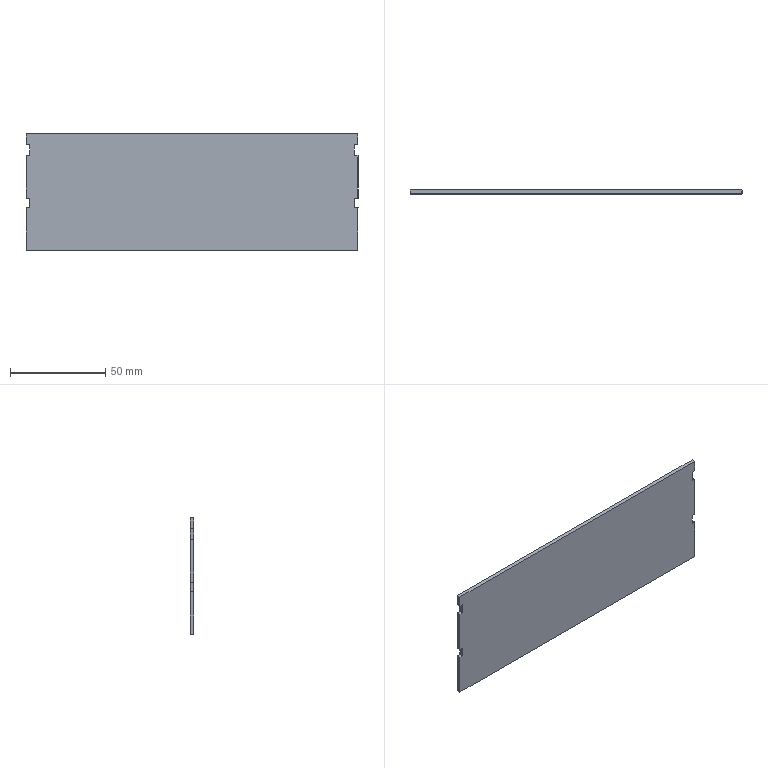Part | SolidWorks | features MirrorStock 1 | 1 solid | 22 faces | box 174 x 2 x 61 mm | volume 21144 mm3 | plane 22
STEP:
#1=CARTESIAN_POINT('',(-87.,-39.2,-39.75));
#2=VERTEX_POINT('',#1);
#3=CARTESIAN_POINT('',(-87.,-41.2,-39.75));
#4=VERTEX_POINT('',#3);
#5=CARTESIAN_POINT('',(-87.,-40.2,-39.75));
#6=DIRECTION('',(0.,-1.,0.));
#7=VECTOR('',#6,1000.);
#8=LINE('',#5,#7);
#9=EDGE_CURVE('',#2,#4,#8,.T.);
#10=ORIENTED_EDGE('',*,*,#9,.T.);
#11=CARTESIAN_POINT('',(-85.,-41.2,-39.75));
#12=VERTEX_POINT('',#11);
#13=CARTESIAN_POINT('',(0.,-41.2,-39.75));
#14=DIRECTION('',(1.,0.,0.));
#15=VECTOR('',#14,1000.);
#16=LINE('',#13,#15);
#17=EDGE_CURVE('',#4,#12,#16,.T.);
#18=ORIENTED_EDGE('',*,*,#17,.T.);
#19=CARTESIAN_POINT('',(-85.,-39.2,-39.75));
#20=VERTEX_POINT('',#19);
#21=CARTESIAN_POINT('',(-85.,-40.2,-39.75));
#22=DIRECTION('',(0.,1.,0.));
#23=VECTOR('',#22,1000.);
#24=LINE('',#21,#23);
#25=EDGE_CURVE('',#12,#20,#24,.T.);
#26=ORIENTED_EDGE('',*,*,#25,.T.);
#27=CARTESIAN_POINT('',(0.,-39.2,-39.75));
#28=DIRECTION('',(-1.,0.,0.));
#29=VECTOR('',#28,1000.);
#30=LINE('',#27,#29);
#31=EDGE_CURVE('',#20,#2,#30,.T.);
#32=ORIENTED_EDGE('',*,*,#31,.T.);
#33=EDGE_LOOP('',(#10,#18,#26,#32));
#34=FACE_OUTER_BOUND('',#33,.T.);
#35=CARTESIAN_POINT('',(-84.779,-38.979,-39.75));
#36=DIRECTION('',(0.,0.,1.));
#37=DIRECTION('',(0.,-1.,0.));
#38=AXIS2_PLACEMENT_3D('',#35,#36,#37);
#39=PLANE('',#38);
#40=ADVANCED_FACE('',(#34),#39,.T.);
#41=CARTESIAN_POINT('',(-85.,-41.2,-34.75));
#42=VERTEX_POINT('',#41);
#43=CARTESIAN_POINT('',(-85.,-39.2,-34.75));
#44=VERTEX_POINT('',#43);
#45=CARTESIAN_POINT('',(-85.,-40.2,-34.75));
#46=DIRECTION('',(0.,1.,0.));
#47=VECTOR('',#46,1000.);
#48=LINE('',#45,#47);
#49=EDGE_CURVE('',#42,#44,#48,.T.);
#50=ORIENTED_EDGE('',*,*,#49,.T.);
#51=CARTESIAN_POINT('',(-85.,-39.2,-31.5));
#52=DIRECTION('',(0.,0.,-1.));
#53=VECTOR('',#52,1000.);
#54=LINE('',#51,#53);
#55=EDGE_CURVE('',#44,#20,#54,.T.);
#56=ORIENTED_EDGE('',*,*,#55,.T.);
#57=ORIENTED_EDGE('',*,*,#25,.F.);
#58=CARTESIAN_POINT('',(-85.,-41.2,-31.5));
#59=DIRECTION('',(0.,0.,1.));
#60=VECTOR('',#59,1000.);
#61=LINE('',#58,#60);
#62=EDGE_CURVE('',#12,#42,#61,.T.);
#63=ORIENTED_EDGE('',*,*,#62,.T.);
#64=EDGE_LOOP('',(#50,#56,#57,#63));
#65=FACE_OUTER_BOUND('',#64,.T.);
#66=CARTESIAN_POINT('',(-85.,-41.421,-34.529));
#67=DIRECTION('',(-1.,0.,0.));
#68=DIRECTION('',(0.,0.,-1.));
#69=AXIS2_PLACEMENT_3D('',#66,#67,#68);
#70=PLANE('',#69);
#71=ADVANCED_FACE('',(#65),#70,.T.);
#72=CARTESIAN_POINT('',(-87.,-41.2,-34.75));
#73=VERTEX_POINT('',#72);
#74=CARTESIAN_POINT('',(-87.,-39.2,-34.75));
#75=VERTEX_POINT('',#74);
#76=CARTESIAN_POINT('',(-87.,-40.2,-34.75));
#77=DIRECTION('',(0.,1.,0.));
#78=VECTOR('',#77,1000.);
#79=LINE('',#76,#78);
#80=EDGE_CURVE('',#73,#75,#79,.T.);
#81=ORIENTED_EDGE('',*,*,#80,.T.);
#82=CARTESIAN_POINT('',(0.,-39.2,-34.75));
#83=DIRECTION('',(1.,0.,0.));
#84=VECTOR('',#83,1000.);
#85=LINE('',#82,#84);
#86=EDGE_CURVE('',#75,#44,#85,.T.);
#87=ORIENTED_EDGE('',*,*,#86,.T.);
#88=ORIENTED_EDGE('',*,*,#49,.F.);
#89=CARTESIAN_POINT('',(0.,-41.2,-34.75));
#90=DIRECTION('',(-1.,0.,0.));
#91=VECTOR('',#90,1000.);
#92=LINE('',#89,#91);
#93=EDGE_CURVE('',#42,#73,#92,.T.);
#94=ORIENTED_EDGE('',*,*,#93,.T.);
#95=EDGE_LOOP('',(#81,#87,#88,#94));
#96=FACE_OUTER_BOUND('',#95,.T.);
#97=CARTESIAN_POINT('',(-84.779,-41.421,-34.75));
#98=DIRECTION('',(0.,0.,-1.));
#99=DIRECTION('',(0.,1.,0.));
#100=AXIS2_PLACEMENT_3D('',#97,#98,#99);
#101=PLANE('',#100);
#102=ADVANCED_FACE('',(#96),#101,.T.);
#103=CARTESIAN_POINT('',(-87.,-41.2,-12.25));
#104=VERTEX_POINT('',#103);
#105=CARTESIAN_POINT('',(-87.,-39.2,-12.25));
#106=VERTEX_POINT('',#105);
#107=CARTESIAN_POINT('',(-87.,-40.2,-12.25));
#108=DIRECTION('',(0.,1.,0.));
#109=VECTOR('',#108,1000.);
#110=LINE('',#107,#109);
#111=EDGE_CURVE('',#104,#106,#110,.T.);
#112=ORIENTED_EDGE('',*,*,#111,.T.);
#113=CARTESIAN_POINT('',(-87.,-39.2,-31.5));
#114=DIRECTION('',(0.,0.,-1.));
#115=VECTOR('',#114,1000.);
#116=LINE('',#113,#115);
#117=EDGE_CURVE('',#106,#75,#116,.T.);
#118=ORIENTED_EDGE('',*,*,#117,.T.);
#119=ORIENTED_EDGE('',*,*,#80,.F.);
#120=CARTESIAN_POINT('',(-87.,-41.2,-31.5));
#121=DIRECTION('',(0.,0.,1.));
#122=VECTOR('',#121,1000.);
#123=LINE('',#120,#122);
#124=EDGE_CURVE('',#73,#104,#123,.T.);
#125=ORIENTED_EDGE('',*,*,#124,.T.);
#126=EDGE_LOOP('',(#112,#118,#119,#125));
#127=FACE_OUTER_BOUND('',#126,.T.);
#128=CARTESIAN_POINT('',(-87.,-41.421,-63.22));
#129=DIRECTION('',(-1.,0.,0.));
#130=DIRECTION('',(0.,1.,0.));
#131=AXIS2_PLACEMENT_3D('',#128,#129,#130);
#132=PLANE('',#131);
#133=ADVANCED_FACE('',(#127),#132,.T.);
#134=CARTESIAN_POINT('',(-85.,-41.2,-12.25));
#135=VERTEX_POINT('',#134);
#136=CARTESIAN_POINT('',(-85.,-39.2,-12.25));
#137=VERTEX_POINT('',#136);
#138=CARTESIAN_POINT('',(-85.,-40.2,-12.25));
#139=DIRECTION('',(0.,1.,0.));
#140=VECTOR('',#139,1000.);
#141=LINE('',#138,#140);
#142=EDGE_CURVE('',#135,#137,#141,.T.);
#143=ORIENTED_EDGE('',*,*,#142,.T.);
#144=CARTESIAN_POINT('',(0.,-39.2,-12.25));
#145=DIRECTION('',(-1.,0.,0.));
#146=VECTOR('',#145,1000.);
#147=LINE('',#144,#146);
#148=EDGE_CURVE('',#137,#106,#147,.T.);
#149=ORIENTED_EDGE('',*,*,#148,.T.);
#150=ORIENTED_EDGE('',*,*,#111,.F.);
#151=CARTESIAN_POINT('',(0.,-41.2,-12.25));
#152=DIRECTION('',(1.,0.,0.));
#153=VECTOR('',#152,1000.);
#154=LINE('',#151,#153);
#155=EDGE_CURVE('',#104,#135,#154,.T.);
#156=ORIENTED_EDGE('',*,*,#155,.T.);
#157=EDGE_LOOP('',(#143,#149,#150,#156));
#158=FACE_OUTER_BOUND('',#157,.T.);
#159=CARTESIAN_POINT('',(-84.779,-38.979,-12.25));
#160=DIRECTION('',(0.,0.,1.));
#161=DIRECTION('',(0.,-1.,0.));
#162=AXIS2_PLACEMENT_3D('',#159,#160,#161);
#163=PLANE('',#162);
#164=ADVANCED_FACE('',(#158),#163,.T.);
#165=CARTESIAN_POINT('',(-85.,-41.2,-6.75));
#166=VERTEX_POINT('',#165);
#167=CARTESIAN_POINT('',(-85.,-41.2,-31.5));
#168=DIRECTION('',(0.,0.,1.));
#169=VECTOR('',#168,1000.);
#170=LINE('',#167,#169);
#171=EDGE_CURVE('',#135,#166,#170,.T.);
#172=ORIENTED_EDGE('',*,*,#171,.T.);
#173=CARTESIAN_POINT('',(-85.,-39.2,-6.75));
#174=VERTEX_POINT('',#173);
#175=CARTESIAN_POINT('',(-85.,-40.2,-6.75));
#176=DIRECTION('',(0.,1.,0.));
#177=VECTOR('',#176,1000.);
#178=LINE('',#175,#177);
#179=EDGE_CURVE('',#166,#174,#178,.T.);
#180=ORIENTED_EDGE('',*,*,#179,.T.);
#181=CARTESIAN_POINT('',(-85.,-39.2,-31.5));
#182=DIRECTION('',(0.,0.,-1.));
#183=VECTOR('',#182,1000.);
#184=LINE('',#181,#183);
#185=EDGE_CURVE('',#174,#137,#184,.T.);
#186=ORIENTED_EDGE('',*,*,#185,.T.);
#187=ORIENTED_EDGE('',*,*,#142,.F.);
#188=EDGE_LOOP('',(#172,#180,#186,#187));
#189=FACE_OUTER_BOUND('',#188,.T.);
#190=CARTESIAN_POINT('',(-85.,-41.421,-6.529));
#191=DIRECTION('',(-1.,0.,0.));
#192=DIRECTION('',(0.,0.,-1.));
#193=AXIS2_PLACEMENT_3D('',#190,#191,#192);
#194=PLANE('',#193);
#195=ADVANCED_FACE('',(#189),#194,.T.);
#196=ORIENTED_EDGE('',*,*,#179,.F.);
#197=CARTESIAN_POINT('',(-87.,-41.2,-6.75));
#198=VERTEX_POINT('',#197);
#199=CARTESIAN_POINT('',(0.,-41.2,-6.75));
#200=DIRECTION('',(-1.,0.,0.));
#201=VECTOR('',#200,1000.);
#202=LINE('',#199,#201);
#203=EDGE_CURVE('',#166,#198,#202,.T.);
#204=ORIENTED_EDGE('',*,*,#203,.T.);
#205=CARTESIAN_POINT('',(-87.,-39.2,-6.75));
#206=VERTEX_POINT('',#205);
#207=CARTESIAN_POINT('',(-87.,-40.2,-6.75));
#208=DIRECTION('',(0.,1.,0.));
#209=VECTOR('',#208,1000.);
#210=LINE('',#207,#209);
#211=EDGE_CURVE('',#198,#206,#210,.T.);
#212=ORIENTED_EDGE('',*,*,#211,.T.);
#213=CARTESIAN_POINT('',(0.,-39.2,-6.75));
#214=DIRECTION('',(1.,0.,0.));
#215=VECTOR('',#214,1000.);
#216=LINE('',#213,#215);
#217=EDGE_CURVE('',#206,#174,#216,.T.);
#218=ORIENTED_EDGE('',*,*,#217,.T.);
#219=EDGE_LOOP('',(#196,#204,#212,#218));
#220=FACE_OUTER_BOUND('',#219,.T.);
#221=CARTESIAN_POINT('',(-84.779,-41.421,-6.75));
#222=DIRECTION('',(0.,0.,-1.));
#223=DIRECTION('',(0.,1.,0.));
#224=AXIS2_PLACEMENT_3D('',#221,#222,#223);
#225=PLANE('',#224);
#226=ADVANCED_FACE('',(#220),#225,.T.);
#227=CARTESIAN_POINT('',(87.,-41.2,-6.75));
#228=VERTEX_POINT('',#227);
#229=CARTESIAN_POINT('',(85.,-41.2,-6.75));
#230=VERTEX_POINT('',#229);
#231=CARTESIAN_POINT('',(0.,-41.2,-6.75));
#232=DIRECTION('',(-1.,0.,0.));
#233=VECTOR('',#232,1000.);
#234=LINE('',#231,#233);
#235=EDGE_CURVE('',#228,#230,#234,.T.);
#236=ORIENTED_EDGE('',*,*,#235,.T.);
#237=CARTESIAN_POINT('',(85.,-39.2,-6.75));
#238=VERTEX_POINT('',#237);
#239=CARTESIAN_POINT('',(85.,-40.2,-6.75));
#240=DIRECTION('',(0.,-1.,0.));
#241=VECTOR('',#240,1000.);
#242=LINE('',#239,#241);
#243=EDGE_CURVE('',#238,#230,#242,.T.);
#244=ORIENTED_EDGE('',*,*,#243,.F.);
#245=CARTESIAN_POINT('',(87.,-39.2,-6.75));
#246=VERTEX_POINT('',#245);
#247=CARTESIAN_POINT('',(0.,-39.2,-6.75));
#248=DIRECTION('',(1.,0.,0.));
#249=VECTOR('',#248,1000.);
#250=LINE('',#247,#249);
#251=EDGE_CURVE('',#238,#246,#250,.T.);
#252=ORIENTED_EDGE('',*,*,#251,.T.);
#253=CARTESIAN_POINT('',(87.,-40.2,-6.75));
#254=DIRECTION('',(0.,-1.,0.));
#255=VECTOR('',#254,1000.);
#256=LINE('',#253,#255);
#257=EDGE_CURVE('',#246,#228,#256,.T.);
#258=ORIENTED_EDGE('',*,*,#257,.T.);
#259=EDGE_LOOP('',(#236,#244,#252,#258));
#260=FACE_OUTER_BOUND('',#259,.T.);
#261=CARTESIAN_POINT('',(84.779,-41.421,-6.75));
#262=DIRECTION('',(0.,0.,1.));
#263=DIRECTION('',(0.,1.,0.));
#264=AXIS2_PLACEMENT_3D('',#261,#262,#263);
#265=PLANE('',#264);
#266=ADVANCED_FACE('',(#260),#265,.F.);
#267=CARTESIAN_POINT('',(85.,-41.2,-12.25));
#268=VERTEX_POINT('',#267);
#269=CARTESIAN_POINT('',(85.,-41.2,-31.5));
#270=DIRECTION('',(0.,0.,-1.));
#271=VECTOR('',#270,1000.);
#272=LINE('',#269,#271);
#273=EDGE_CURVE('',#230,#268,#272,.T.);
#274=ORIENTED_EDGE('',*,*,#273,.T.);
#275=CARTESIAN_POINT('',(85.,-39.2,-12.25));
#276=VERTEX_POINT('',#275);
#277=CARTESIAN_POINT('',(85.,-40.2,-12.25));
#278=DIRECTION('',(0.,-1.,0.));
#279=VECTOR('',#278,1000.);
#280=LINE('',#277,#279);
#281=EDGE_CURVE('',#276,#268,#280,.T.);
#282=ORIENTED_EDGE('',*,*,#281,.F.);
#283=CARTESIAN_POINT('',(85.,-39.2,-31.5));
#284=DIRECTION('',(0.,0.,1.));
#285=VECTOR('',#284,1000.);
#286=LINE('',#283,#285);
#287=EDGE_CURVE('',#276,#238,#286,.T.);
#288=ORIENTED_EDGE('',*,*,#287,.T.);
#289=ORIENTED_EDGE('',*,*,#243,.T.);
#290=EDGE_LOOP('',(#274,#282,#288,#289));
#291=FACE_OUTER_BOUND('',#290,.T.);
#292=CARTESIAN_POINT('',(85.,-41.421,-6.529));
#293=DIRECTION('',(-1.,0.,0.));
#294=DIRECTION('',(0.,0.,-1.));
#295=AXIS2_PLACEMENT_3D('',#292,#293,#294);
#296=PLANE('',#295);
#297=ADVANCED_FACE('',(#291),#296,.F.);
#298=CARTESIAN_POINT('',(87.,-41.2,-12.25));
#299=VERTEX_POINT('',#298);
#300=CARTESIAN_POINT('',(0.,-41.2,-12.25));
#301=DIRECTION('',(1.,0.,0.));
#302=VECTOR('',#301,1000.);
#303=LINE('',#300,#302);
#304=EDGE_CURVE('',#268,#299,#303,.T.);
#305=ORIENTED_EDGE('',*,*,#304,.T.);
#306=CARTESIAN_POINT('',(87.,-39.2,-12.25));
#307=VERTEX_POINT('',#306);
#308=CARTESIAN_POINT('',(87.,-40.2,-12.25));
#309=DIRECTION('',(0.,1.,0.));
#310=VECTOR('',#309,1000.);
#311=LINE('',#308,#310);
#312=EDGE_CURVE('',#299,#307,#311,.T.);
#313=ORIENTED_EDGE('',*,*,#312,.T.);
#314=CARTESIAN_POINT('',(0.,-39.2,-12.25));
#315=DIRECTION('',(-1.,0.,0.));
#316=VECTOR('',#315,1000.);
#317=LINE('',#314,#316);
#318=EDGE_CURVE('',#307,#276,#317,.T.);
#319=ORIENTED_EDGE('',*,*,#318,.T.);
#320=ORIENTED_EDGE('',*,*,#281,.T.);
#321=EDGE_LOOP('',(#305,#313,#319,#320));
#322=FACE_OUTER_BOUND('',#321,.T.);
#323=CARTESIAN_POINT('',(84.779,-38.979,-12.25));
#324=DIRECTION('',(0.,0.,-1.));
#325=DIRECTION('',(0.,-1.,0.));
#326=AXIS2_PLACEMENT_3D('',#323,#324,#325);
#327=PLANE('',#326);
#328=ADVANCED_FACE('',(#322),#327,.F.);
#329=ORIENTED_EDGE('',*,*,#312,.F.);
#330=CARTESIAN_POINT('',(87.,-41.2,-34.75));
#331=VERTEX_POINT('',#330);
#332=CARTESIAN_POINT('',(87.,-41.2,-31.5));
#333=DIRECTION('',(0.,0.,-1.));
#334=VECTOR('',#333,1000.);
#335=LINE('',#332,#334);
#336=EDGE_CURVE('',#299,#331,#335,.T.);
#337=ORIENTED_EDGE('',*,*,#336,.T.);
#338=CARTESIAN_POINT('',(87.,-39.2,-34.75));
#339=VERTEX_POINT('',#338);
#340=CARTESIAN_POINT('',(87.,-40.2,-34.75));
#341=DIRECTION('',(0.,-1.,0.));
#342=VECTOR('',#341,1000.);
#343=LINE('',#340,#342);
#344=EDGE_CURVE('',#339,#331,#343,.T.);
#345=ORIENTED_EDGE('',*,*,#344,.F.);
#346=CARTESIAN_POINT('',(87.,-39.2,-31.5));
#347=DIRECTION('',(0.,0.,1.));
#348=VECTOR('',#347,1000.);
#349=LINE('',#346,#348);
#350=EDGE_CURVE('',#339,#307,#349,.T.);
#351=ORIENTED_EDGE('',*,*,#350,.T.);
#352=EDGE_LOOP('',(#329,#337,#345,#351));
#353=FACE_OUTER_BOUND('',#352,.T.);
#354=CARTESIAN_POINT('',(87.,-38.979,-63.22));
#355=DIRECTION('',(1.,0.,0.));
#356=DIRECTION('',(0.,-1.,0.));
#357=AXIS2_PLACEMENT_3D('',#354,#355,#356);
#358=PLANE('',#357);
#359=ADVANCED_FACE('',(#353),#358,.T.);
#360=CARTESIAN_POINT('',(85.,-41.2,-34.75));
#361=VERTEX_POINT('',#360);
#362=CARTESIAN_POINT('',(0.,-41.2,-34.75));
#363=DIRECTION('',(-1.,0.,0.));
#364=VECTOR('',#363,1000.);
#365=LINE('',#362,#364);
#366=EDGE_CURVE('',#331,#361,#365,.T.);
#367=ORIENTED_EDGE('',*,*,#366,.T.);
#368=CARTESIAN_POINT('',(85.,-39.2,-34.75));
#369=VERTEX_POINT('',#368);
#370=CARTESIAN_POINT('',(85.,-40.2,-34.75));
#371=DIRECTION('',(0.,-1.,0.));
#372=VECTOR('',#371,1000.);
#373=LINE('',#370,#372);
#374=EDGE_CURVE('',#369,#361,#373,.T.);
#375=ORIENTED_EDGE('',*,*,#374,.F.);
#376=CARTESIAN_POINT('',(0.,-39.2,-34.75));
#377=DIRECTION('',(1.,0.,0.));
#378=VECTOR('',#377,1000.);
#379=LINE('',#376,#378);
#380=EDGE_CURVE('',#369,#339,#379,.T.);
#381=ORIENTED_EDGE('',*,*,#380,.T.);
#382=ORIENTED_EDGE('',*,*,#344,.T.);
#383=EDGE_LOOP('',(#367,#375,#381,#382));
#384=FACE_OUTER_BOUND('',#383,.T.);
#385=CARTESIAN_POINT('',(84.779,-41.421,-34.75));
#386=DIRECTION('',(0.,0.,1.));
#387=DIRECTION('',(0.,1.,0.));
#388=AXIS2_PLACEMENT_3D('',#385,#386,#387);
#389=PLANE('',#388);
#390=ADVANCED_FACE('',(#384),#389,.F.);
#391=CARTESIAN_POINT('',(85.,-41.2,-39.75));
#392=VERTEX_POINT('',#391);
#393=CARTESIAN_POINT('',(85.,-41.2,-31.5));
#394=DIRECTION('',(0.,0.,-1.));
#395=VECTOR('',#394,1000.);
#396=LINE('',#393,#395);
#397=EDGE_CURVE('',#361,#392,#396,.T.);
#398=ORIENTED_EDGE('',*,*,#397,.T.);
#399=CARTESIAN_POINT('',(85.,-39.2,-39.75));
#400=VERTEX_POINT('',#399);
#401=CARTESIAN_POINT('',(85.,-40.2,-39.75));
#402=DIRECTION('',(0.,-1.,0.));
#403=VECTOR('',#402,1000.);
#404=LINE('',#401,#403);
#405=EDGE_CURVE('',#400,#392,#404,.T.);
#406=ORIENTED_EDGE('',*,*,#405,.F.);
#407=CARTESIAN_POINT('',(85.,-39.2,-31.5));
#408=DIRECTION('',(0.,0.,1.));
#409=VECTOR('',#408,1000.);
#410=LINE('',#407,#409);
#411=EDGE_CURVE('',#400,#369,#410,.T.);
#412=ORIENTED_EDGE('',*,*,#411,.T.);
#413=ORIENTED_EDGE('',*,*,#374,.T.);
#414=EDGE_LOOP('',(#398,#406,#412,#413));
#415=FACE_OUTER_BOUND('',#414,.T.);
#416=CARTESIAN_POINT('',(85.,-41.421,-34.529));
#417=DIRECTION('',(-1.,0.,0.));
#418=DIRECTION('',(0.,0.,-1.));
#419=AXIS2_PLACEMENT_3D('',#416,#417,#418);
#420=PLANE('',#419);
#421=ADVANCED_FACE('',(#415),#420,.F.);
#422=CARTESIAN_POINT('',(87.,-41.2,-39.75));
#423=VERTEX_POINT('',#422);
#424=CARTESIAN_POINT('',(0.,-41.2,-39.75));
#425=DIRECTION('',(1.,0.,0.));
#426=VECTOR('',#425,1000.);
#427=LINE('',#424,#426);
#428=EDGE_CURVE('',#392,#423,#427,.T.);
#429=ORIENTED_EDGE('',*,*,#428,.T.);
#430=CARTESIAN_POINT('',(87.,-39.2,-39.75));
#431=VERTEX_POINT('',#430);
#432=CARTESIAN_POINT('',(87.,-40.2,-39.75));
#433=DIRECTION('',(0.,1.,0.));
#434=VECTOR('',#433,1000.);
#435=LINE('',#432,#434);
#436=EDGE_CURVE('',#423,#431,#435,.T.);
#437=ORIENTED_EDGE('',*,*,#436,.T.);
#438=CARTESIAN_POINT('',(0.,-39.2,-39.75));
#439=DIRECTION('',(-1.,0.,0.));
#440=VECTOR('',#439,1000.);
#441=LINE('',#438,#440);
#442=EDGE_CURVE('',#431,#400,#441,.T.);
#443=ORIENTED_EDGE('',*,*,#442,.T.);
#444=ORIENTED_EDGE('',*,*,#405,.T.);
#445=EDGE_LOOP('',(#429,#437,#443,#444));
#446=FACE_OUTER_BOUND('',#445,.T.);
#447=CARTESIAN_POINT('',(84.779,-38.979,-39.75));
#448=DIRECTION('',(0.,0.,-1.));
#449=DIRECTION('',(0.,-1.,0.));
#450=AXIS2_PLACEMENT_3D('',#447,#448,#449);
#451=PLANE('',#450);
#452=ADVANCED_FACE('',(#446),#451,.F.);
#453=CARTESIAN_POINT('',(87.,-39.2,-62.));
#454=VERTEX_POINT('',#453);
#455=CARTESIAN_POINT('',(87.,-41.2,-62.));
#456=VERTEX_POINT('',#455);
#457=CARTESIAN_POINT('',(87.,-40.2,-62.));
#458=DIRECTION('',(0.,-1.,0.));
#459=VECTOR('',#458,1000.);
#460=LINE('',#457,#459);
#461=EDGE_CURVE('',#454,#456,#460,.T.);
#462=ORIENTED_EDGE('',*,*,#461,.F.);
#463=CARTESIAN_POINT('',(87.,-39.2,-31.5));
#464=DIRECTION('',(0.,0.,1.));
#465=VECTOR('',#464,1000.);
#466=LINE('',#463,#465);
#467=EDGE_CURVE('',#454,#431,#466,.T.);
#468=ORIENTED_EDGE('',*,*,#467,.T.);
#469=ORIENTED_EDGE('',*,*,#436,.F.);
#470=CARTESIAN_POINT('',(87.,-41.2,-31.5));
#471=DIRECTION('',(0.,0.,-1.));
#472=VECTOR('',#471,1000.);
#473=LINE('',#470,#472);
#474=EDGE_CURVE('',#423,#456,#473,.T.);
#475=ORIENTED_EDGE('',*,*,#474,.T.);
#476=EDGE_LOOP('',(#462,#468,#469,#475));
#477=FACE_OUTER_BOUND('',#476,.T.);
#478=CARTESIAN_POINT('',(87.,-38.979,-63.22));
#479=DIRECTION('',(1.,0.,0.));
#480=DIRECTION('',(0.,-1.,0.));
#481=AXIS2_PLACEMENT_3D('',#478,#479,#480);
#482=PLANE('',#481);
#483=ADVANCED_FACE('',(#477),#482,.T.);
#484=ORIENTED_EDGE('',*,*,#461,.T.);
#485=CARTESIAN_POINT('',(-87.,-41.2,-62.));
#486=VERTEX_POINT('',#485);
#487=CARTESIAN_POINT('',(0.,-41.2,-62.));
#488=DIRECTION('',(-1.,0.,0.));
#489=VECTOR('',#488,1000.);
#490=LINE('',#487,#489);
#491=EDGE_CURVE('',#456,#486,#490,.T.);
#492=ORIENTED_EDGE('',*,*,#491,.T.);
#493=CARTESIAN_POINT('',(-87.,-39.2,-62.));
#494=VERTEX_POINT('',#493);
#495=CARTESIAN_POINT('',(-87.,-40.2,-62.));
#496=DIRECTION('',(0.,1.,0.));
#497=VECTOR('',#496,1000.);
#498=LINE('',#495,#497);
#499=EDGE_CURVE('',#486,#494,#498,.T.);
#500=ORIENTED_EDGE('',*,*,#499,.T.);
#501=CARTESIAN_POINT('',(0.,-39.2,-62.));
#502=DIRECTION('',(1.,0.,0.));
#503=VECTOR('',#502,1000.);
#504=LINE('',#501,#503);
#505=EDGE_CURVE('',#494,#454,#504,.T.);
#506=ORIENTED_EDGE('',*,*,#505,.T.);
#507=EDGE_LOOP('',(#484,#492,#500,#506));
#508=FACE_OUTER_BOUND('',#507,.T.);
#509=CARTESIAN_POINT('',(90.48,-38.979,-62.));
#510=DIRECTION('',(0.,0.,1.));
#511=DIRECTION('',(0.,-1.,0.));
#512=AXIS2_PLACEMENT_3D('',#509,#510,#511);
#513=PLANE('',#512);
#514=ADVANCED_FACE('',(#508),#513,.F.);
#515=ORIENTED_EDGE('',*,*,#499,.F.);
#516=CARTESIAN_POINT('',(-87.,-41.2,-31.5));
#517=DIRECTION('',(0.,0.,1.));
#518=VECTOR('',#517,1000.);
#519=LINE('',#516,#518);
#520=EDGE_CURVE('',#486,#4,#519,.T.);
#521=ORIENTED_EDGE('',*,*,#520,.T.);
#522=ORIENTED_EDGE('',*,*,#9,.F.);
#523=CARTESIAN_POINT('',(-87.,-39.2,-31.5));
#524=DIRECTION('',(0.,0.,-1.));
#525=VECTOR('',#524,1000.);
#526=LINE('',#523,#525);
#527=EDGE_CURVE('',#2,#494,#526,.T.);
#528=ORIENTED_EDGE('',*,*,#527,.T.);
#529=EDGE_LOOP('',(#515,#521,#522,#528));
#530=FACE_OUTER_BOUND('',#529,.T.);
#531=CARTESIAN_POINT('',(-87.,-41.421,-63.22));
#532=DIRECTION('',(-1.,0.,0.));
#533=DIRECTION('',(0.,1.,0.));
#534=AXIS2_PLACEMENT_3D('',#531,#532,#533);
#535=PLANE('',#534);
#536=ADVANCED_FACE('',(#530),#535,.T.);
#537=CARTESIAN_POINT('',(-87.,-39.2,-1.));
#538=VERTEX_POINT('',#537);
#539=CARTESIAN_POINT('',(-87.,-39.2,-31.5));
#540=DIRECTION('',(0.,0.,-1.));
#541=VECTOR('',#540,1000.);
#542=LINE('',#539,#541);
#543=EDGE_CURVE('',#538,#206,#542,.T.);
#544=ORIENTED_EDGE('',*,*,#543,.T.);
#545=ORIENTED_EDGE('',*,*,#211,.F.);
#546=CARTESIAN_POINT('',(-87.,-41.2,-1.));
#547=VERTEX_POINT('',#546);
#548=CARTESIAN_POINT('',(-87.,-41.2,-31.5));
#549=DIRECTION('',(0.,0.,1.));
#550=VECTOR('',#549,1000.);
#551=LINE('',#548,#550);
#552=EDGE_CURVE('',#198,#547,#551,.T.);
#553=ORIENTED_EDGE('',*,*,#552,.T.);
#554=CARTESIAN_POINT('',(-87.,-40.2,-1.));
#555=DIRECTION('',(0.,1.,0.));
#556=VECTOR('',#555,1000.);
#557=LINE('',#554,#556);
#558=EDGE_CURVE('',#547,#538,#557,.T.);
#559=ORIENTED_EDGE('',*,*,#558,.T.);
#560=EDGE_LOOP('',(#544,#545,#553,#559));
#561=FACE_OUTER_BOUND('',#560,.T.);
#562=CARTESIAN_POINT('',(-87.,-41.421,-63.22));
#563=DIRECTION('',(-1.,0.,0.));
#564=DIRECTION('',(0.,1.,0.));
#565=AXIS2_PLACEMENT_3D('',#562,#563,#564);
#566=PLANE('',#565);
#567=ADVANCED_FACE('',(#561),#566,.T.);
#568=ORIENTED_EDGE('',*,*,#86,.F.);
#569=ORIENTED_EDGE('',*,*,#117,.F.);
#570=ORIENTED_EDGE('',*,*,#148,.F.);
#571=ORIENTED_EDGE('',*,*,#185,.F.);
#572=ORIENTED_EDGE('',*,*,#217,.F.);
#573=ORIENTED_EDGE('',*,*,#543,.F.);
#574=CARTESIAN_POINT('',(87.,-39.2,-1.));
#575=VERTEX_POINT('',#574);
#576=CARTESIAN_POINT('',(0.,-39.2,-1.));
#577=DIRECTION('',(1.,0.,0.));
#578=VECTOR('',#577,1000.);
#579=LINE('',#576,#578);
#580=EDGE_CURVE('',#538,#575,#579,.T.);
#581=ORIENTED_EDGE('',*,*,#580,.T.);
#582=CARTESIAN_POINT('',(87.,-39.2,-31.5));
#583=DIRECTION('',(0.,0.,-1.));
#584=VECTOR('',#583,1000.);
#585=LINE('',#582,#584);
#586=EDGE_CURVE('',#575,#246,#585,.T.);
#587=ORIENTED_EDGE('',*,*,#586,.T.);
#588=ORIENTED_EDGE('',*,*,#251,.F.);
#589=ORIENTED_EDGE('',*,*,#287,.F.);
#590=ORIENTED_EDGE('',*,*,#318,.F.);
#591=ORIENTED_EDGE('',*,*,#350,.F.);
#592=ORIENTED_EDGE('',*,*,#380,.F.);
#593=ORIENTED_EDGE('',*,*,#411,.F.);
#594=ORIENTED_EDGE('',*,*,#442,.F.);
#595=ORIENTED_EDGE('',*,*,#467,.F.);
#596=ORIENTED_EDGE('',*,*,#505,.F.);
#597=ORIENTED_EDGE('',*,*,#527,.F.);
#598=ORIENTED_EDGE('',*,*,#31,.F.);
#599=ORIENTED_EDGE('',*,*,#55,.F.);
#600=EDGE_LOOP('',(#568,#569,#570,#571,#572,#573,#581,#587,#588,#589,#590,#591,#592,#593,#594,#595,#596,#597,#598,#599));
#601=FACE_OUTER_BOUND('',#600,.T.);
#602=CARTESIAN_POINT('',(-90.48,-39.2,-63.22));
#603=DIRECTION('',(0.,1.,0.));
#604=DIRECTION('',(1.,0.,0.));
#605=AXIS2_PLACEMENT_3D('',#602,#603,#604);
#606=PLANE('',#605);
#607=ADVANCED_FACE('',(#601),#606,.T.);
#608=CARTESIAN_POINT('',(87.,-41.2,-1.));
#609=VERTEX_POINT('',#608);
#610=CARTESIAN_POINT('',(87.,-41.2,-31.5));
#611=DIRECTION('',(0.,0.,-1.));
#612=VECTOR('',#611,1000.);
#613=LINE('',#610,#612);
#614=EDGE_CURVE('',#609,#228,#613,.T.);
#615=ORIENTED_EDGE('',*,*,#614,.T.);
#616=ORIENTED_EDGE('',*,*,#257,.F.);
#617=ORIENTED_EDGE('',*,*,#586,.F.);
#618=CARTESIAN_POINT('',(87.,-40.2,-1.));
#619=DIRECTION('',(0.,-1.,0.));
#620=VECTOR('',#619,1000.);
#621=LINE('',#618,#620);
#622=EDGE_CURVE('',#575,#609,#621,.T.);
#623=ORIENTED_EDGE('',*,*,#622,.T.);
#624=EDGE_LOOP('',(#615,#616,#617,#623));
#625=FACE_OUTER_BOUND('',#624,.T.);
#626=CARTESIAN_POINT('',(87.,-38.979,-63.22));
#627=DIRECTION('',(1.,0.,0.));
#628=DIRECTION('',(0.,-1.,0.));
#629=AXIS2_PLACEMENT_3D('',#626,#627,#628);
#630=PLANE('',#629);
#631=ADVANCED_FACE('',(#625),#630,.T.);
#632=ORIENTED_EDGE('',*,*,#491,.F.);
#633=ORIENTED_EDGE('',*,*,#474,.F.);
#634=ORIENTED_EDGE('',*,*,#428,.F.);
#635=ORIENTED_EDGE('',*,*,#397,.F.);
#636=ORIENTED_EDGE('',*,*,#366,.F.);
#637=ORIENTED_EDGE('',*,*,#336,.F.);
#638=ORIENTED_EDGE('',*,*,#304,.F.);
#639=ORIENTED_EDGE('',*,*,#273,.F.);
#640=ORIENTED_EDGE('',*,*,#235,.F.);
#641=ORIENTED_EDGE('',*,*,#614,.F.);
#642=CARTESIAN_POINT('',(0.,-41.2,-1.));
#643=DIRECTION('',(-1.,0.,0.));
#644=VECTOR('',#643,1000.);
#645=LINE('',#642,#644);
#646=EDGE_CURVE('',#609,#547,#645,.T.);
#647=ORIENTED_EDGE('',*,*,#646,.T.);
#648=ORIENTED_EDGE('',*,*,#552,.F.);
#649=ORIENTED_EDGE('',*,*,#203,.F.);
#650=ORIENTED_EDGE('',*,*,#171,.F.);
#651=ORIENTED_EDGE('',*,*,#155,.F.);
#652=ORIENTED_EDGE('',*,*,#124,.F.);
#653=ORIENTED_EDGE('',*,*,#93,.F.);
#654=ORIENTED_EDGE('',*,*,#62,.F.);
#655=ORIENTED_EDGE('',*,*,#17,.F.);
#656=ORIENTED_EDGE('',*,*,#520,.F.);
#657=EDGE_LOOP('',(#632,#633,#634,#635,#636,#637,#638,#639,#640,#641,#647,#648,#649,#650,#651,#652,#653,#654,#655,#656));
#658=FACE_OUTER_BOUND('',#657,.T.);
#659=CARTESIAN_POINT('',(90.48,-41.2,-63.22));
#660=DIRECTION('',(0.,-1.,0.));
#661=DIRECTION('',(-1.,0.,0.));
#662=AXIS2_PLACEMENT_3D('',#659,#660,#661);
#663=PLANE('',#662);
#664=ADVANCED_FACE('',(#658),#663,.T.);
#665=ORIENTED_EDGE('',*,*,#622,.F.);
#666=ORIENTED_EDGE('',*,*,#580,.F.);
#667=ORIENTED_EDGE('',*,*,#558,.F.);
#668=ORIENTED_EDGE('',*,*,#646,.F.);
#669=EDGE_LOOP('',(#665,#666,#667,#668));
#670=FACE_OUTER_BOUND('',#669,.T.);
#671=CARTESIAN_POINT('',(90.48,-38.979,-1.));
#672=DIRECTION('',(0.,0.,1.));
#673=DIRECTION('',(0.,-1.,0.));
#674=AXIS2_PLACEMENT_3D('',#671,#672,#673);
#675=PLANE('',#674);
#676=ADVANCED_FACE('',(#670),#675,.T.);
#677=CLOSED_SHELL('',(#40,#71,#102,#133,#164,#195,#226,#266,#297,#328,#359,#390,#421,#452,#483,#514,#536,#567,#607,#631,#664,#676));
#678=MANIFOLD_SOLID_BREP('',#677);
#679=CARTESIAN_POINT('',(0.,0.,0.));
#680=DIRECTION('',(0.,0.,1.));
#681=DIRECTION('',(1.,0.,0.));
#682=AXIS2_PLACEMENT_3D('',#679,#680,#681);
#683=(LENGTH_UNIT()NAMED_UNIT(*)SI_UNIT(.MILLI.,.METRE.));
#684=UNCERTAINTY_MEASURE_WITH_UNIT(LENGTH_MEASURE(0.00001),#683,'','');
#685=(NAMED_UNIT(*)PLANE_ANGLE_UNIT()SI_UNIT($,.RADIAN.));
#686=(NAMED_UNIT(*)SI_UNIT($,.STERADIAN.)SOLID_ANGLE_UNIT());
#687=(GEOMETRIC_REPRESENTATION_CONTEXT(3)GLOBAL_UNCERTAINTY_ASSIGNED_CONTEXT((#684))GLOBAL_UNIT_ASSIGNED_CONTEXT((#683,#685,#686))REPRESENTATION_CONTEXT('',''));
#688=ADVANCED_BREP_SHAPE_REPRESENTATION('',(#678,#682),#687);